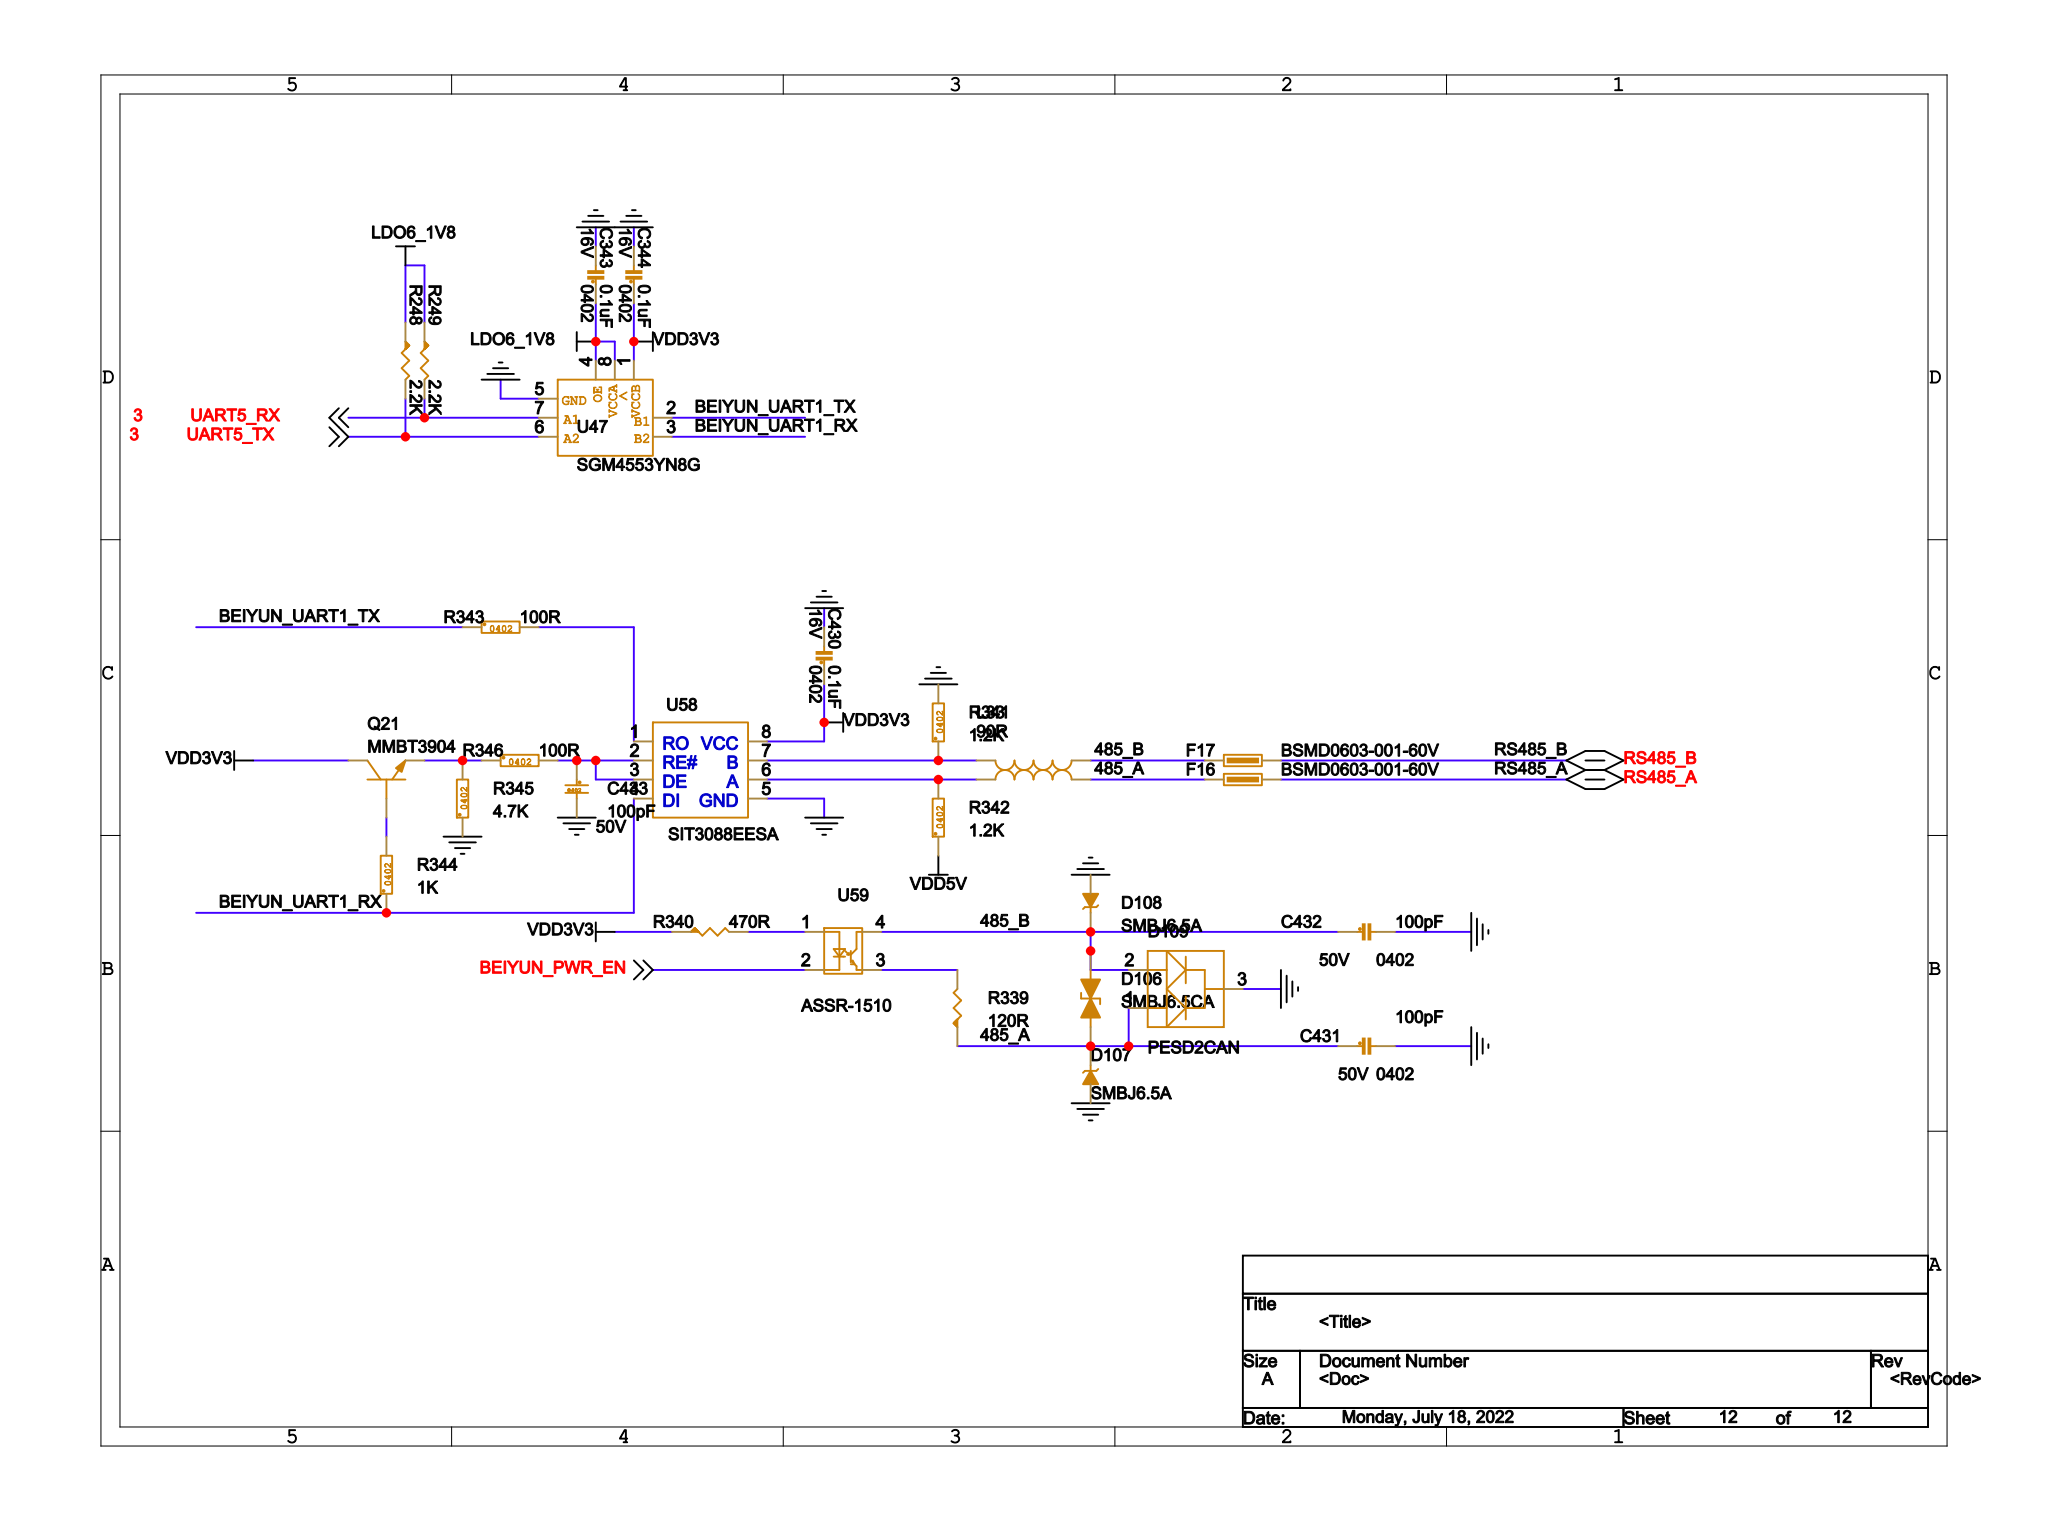Circuit board | Cadence Allegro | 970 parts | 627 nets | one sheet of the schematic
Parts on this sheet (reference | value | footprint):
C343 | 0.1uF | C0402
C344 | 0.1uF | C0402
C430 | 0.1uF | C0402
C431 | 100pF | C0402
C432 | 100pF | C0402
C433 | 100pF | C0402
D106 | SMBJ6.5CA | SMB
D107 | SMBJ6.5A | SMB
D108 | SMBJ6.5A | SMB
D109 | PESD2CAN | SOT-23
F16 | BSMD0603-001-60V | R0603
F17 | BSMD0603-001-60V | R0603
L33 | 90R | WCM2012
Q21 | MMBT3904 | SOT-23
R248 | 2.2K | R0402
R249 | 2.2K | R0402
R339 | 120R | R0603
R340 | 470R | R0402
R341 | 1.2K | R0402
R342 | 1.2K | R0402
R343 | 100R | R0402
R344 | 1K | R0402
R345 | 4.7K | R0402
R346 | 100R | R0402
U47 | SGM4553YN8G | SOT23_8
U58 | SIT3088EESA | SO8
U59 | ASSR-1510 | SO4
Nets of these parts (net: part-pin ...):
VDD5V: R342-1
VDD3V3: C344-1 C430-1 Q21-3 R340-1 U47-1 U58-8
GND: C343-2 C344-2 C430-2 C431-2 C432-2 C433-2 D107-1 D108-1 D109-3 R341-2 R345-1 U47-5 U58-5
LDO6_1V8: C343-1 R248-1 R249-1 U47-4 U47-8
N19763989: Q21-1 R344-2
N19764047: Q21-2 R345-2 R346-1
BEIYUN_UART1_TX: R343-1 U47-2
N19752935: R343-2 U58-1
N19764053: C433-1 R346-2 U58-2 U58-3
N19752416: L33-1 R341-1 U58-7
N19752419: L33-3 R342-2 U58-6
BEIYUN_UART1_RX: R344-1 U47-3 U58-4
485_A: C431-1 D106-1 D107-2 D109-1 F16-1 L33-4 R339-1
485_B: C432-1 D106-2 D108-2 D109-2 F17-1 L33-2 U59-4
RS485_A: F16-2
RS485_B: F17-2
UART5_TX: R248-2 U47-6
UART5_RX: R249-2 U47-7
N19752725: R340-2 U59-1
N19752689: R339-2 U59-3
BEIYUN_PWR_EN: U59-2